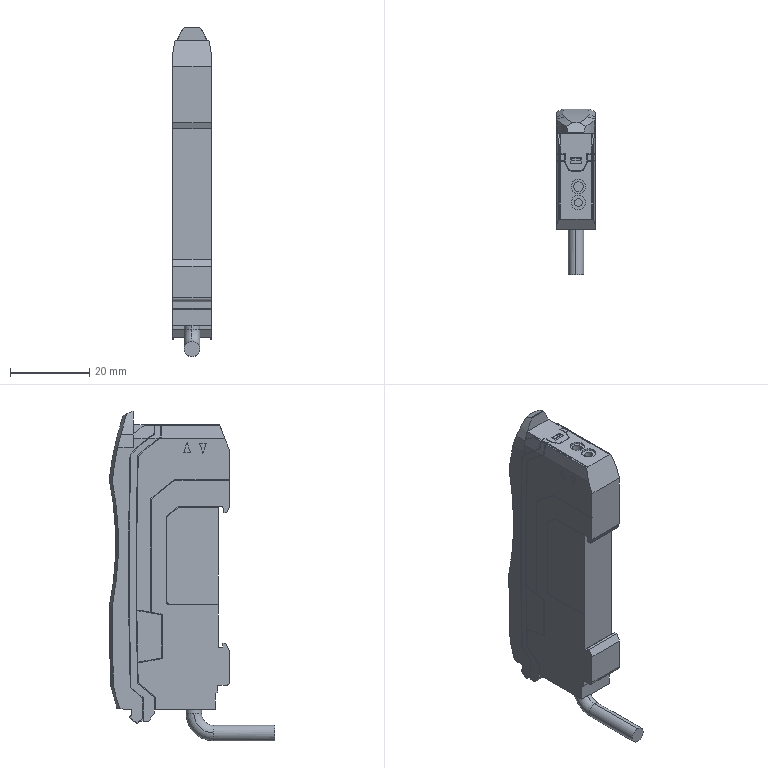Part | NX | 1 solid | 314 faces | box 9.8 x 41.701 x 83.1 mm | volume 19769 mm3 | plane 224 | cylinder 70 | cone 9 | spline 8 | torus 3 | commonest cylinder face diameters 2 x9 1.66 x6 0.6 x4 3.628 x4 3.9 x4 1.601 x2